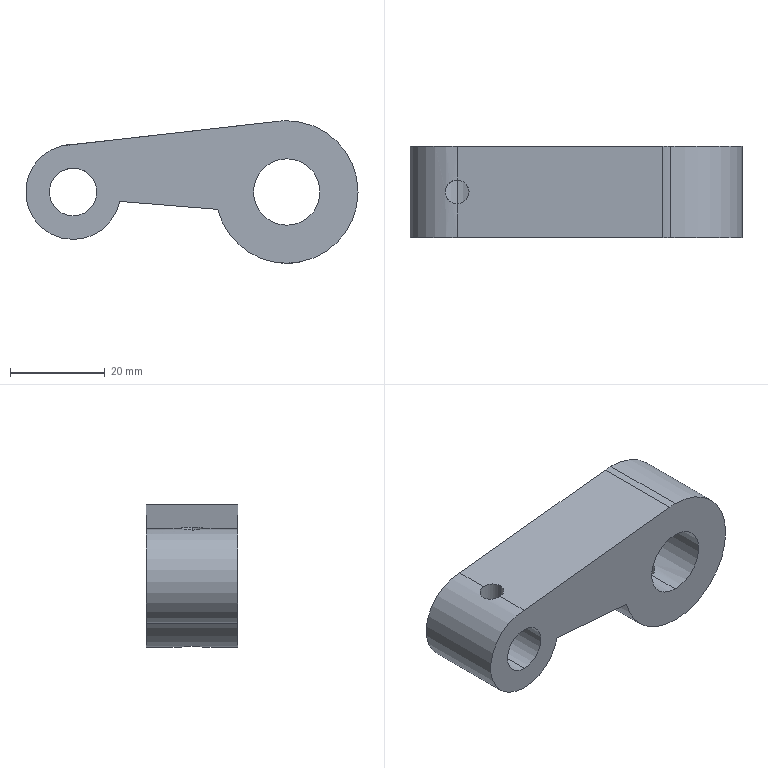Part | SolidWorks | features BaseBody 1 | 1 solid | 17 faces | box 70 x 19.2 x 30 mm | volume 21910 mm3 | cylinder 13 | plane 4 | commonest cylinder face diameters 5 x4 30 x3 10 x2 14 x2 20 x2
STEP:
#1=CARTESIAN_POINT('',(-45.,19.2,10.));
#2=VERTEX_POINT('',#1);
#3=CARTESIAN_POINT('',(-45.,19.2,-10.));
#4=VERTEX_POINT('',#3);
#5=CARTESIAN_POINT('',(-45.,19.2,0.));
#6=DIRECTION('',(0.,-1.,0.));
#7=DIRECTION('',(0.,0.,-1.));
#8=AXIS2_PLACEMENT_3D('',#5,#6,#7);
#9=CIRCLE('',#8,10.);
#10=EDGE_CURVE('',#2,#4,#9,.T.);
#11=ORIENTED_EDGE('',*,*,#10,.T.);
#12=CARTESIAN_POINT('',(-45.,0.,-10.));
#13=VERTEX_POINT('',#12);
#14=CARTESIAN_POINT('',(-45.,19.2,-10.));
#15=DIRECTION('',(0.,-1.,0.));
#16=VECTOR('',#15,1000.);
#17=LINE('',#14,#16);
#18=EDGE_CURVE('',#4,#13,#17,.T.);
#19=ORIENTED_EDGE('',*,*,#18,.T.);
#20=CARTESIAN_POINT('',(-45.,0.,10.));
#21=VERTEX_POINT('',#20);
#22=CARTESIAN_POINT('',(-45.,0.,0.));
#23=DIRECTION('',(0.,1.,0.));
#24=DIRECTION('',(0.,0.,-1.));
#25=AXIS2_PLACEMENT_3D('',#22,#23,#24);
#26=CIRCLE('',#25,10.);
#27=EDGE_CURVE('',#13,#21,#26,.T.);
#28=ORIENTED_EDGE('',*,*,#27,.T.);
#29=CARTESIAN_POINT('',(-45.,7.1,10.));
#30=VERTEX_POINT('',#29);
#31=CARTESIAN_POINT('',(-45.,19.2,10.));
#32=DIRECTION('',(0.,1.,0.));
#33=VECTOR('',#32,1000.);
#34=LINE('',#31,#33);
#35=EDGE_CURVE('',#21,#30,#34,.T.);
#36=ORIENTED_EDGE('',*,*,#35,.T.);
#37=CARTESIAN_POINT('',(-47.5,9.6,9.682));
#38=VERTEX_POINT('',#37);
#39=CARTESIAN_POINT('',(-45.,7.1,10.));
#40=CARTESIAN_POINT('',(-45.166,7.1,10.));
#41=CARTESIAN_POINT('',(-45.329,7.116,9.996));
#42=CARTESIAN_POINT('',(-45.649,7.18,9.98));
#43=CARTESIAN_POINT('',(-45.808,7.229,9.968));
#44=CARTESIAN_POINT('',(-46.11,7.354,9.939));
#45=CARTESIAN_POINT('',(-46.254,7.431,9.922));
#46=CARTESIAN_POINT('',(-46.525,7.612,9.884));
#47=CARTESIAN_POINT('',(-46.653,7.717,9.863));
#48=CARTESIAN_POINT('',(-46.997,8.061,9.801));
#49=CARTESIAN_POINT('',(-47.183,8.339,9.76));
#50=CARTESIAN_POINT('',(-47.37,8.789,9.715));
#51=CARTESIAN_POINT('',(-47.419,8.947,9.703));
#52=CARTESIAN_POINT('',(-47.484,9.27,9.687));
#53=CARTESIAN_POINT('',(-47.5,9.434,9.682));
#54=CARTESIAN_POINT('',(-47.5,9.6,9.682));
#55=B_SPLINE_CURVE_WITH_KNOTS('',3,(#39,#40,#41,#42,#43,#44,#45,#46,#47,#48,#49,#50,#51,#52,#53,#54),.UNSPECIFIED.,.F.,.F.,(4,2,2,2,2,2,2,4),(-0.003921,-0.003431,-0.002941,-0.002451,-0.00196,-0.0009802,-0.0004901,0.),.UNSPECIFIED.);
#56=EDGE_CURVE('',#30,#38,#55,.T.);
#57=ORIENTED_EDGE('',*,*,#56,.T.);
#58=CARTESIAN_POINT('',(-45.,12.1,10.));
#59=VERTEX_POINT('',#58);
#60=CARTESIAN_POINT('',(-47.5,9.6,9.682));
#61=CARTESIAN_POINT('',(-47.5,9.766,9.682));
#62=CARTESIAN_POINT('',(-47.484,9.929,9.687));
#63=CARTESIAN_POINT('',(-47.42,10.249,9.703));
#64=CARTESIAN_POINT('',(-47.372,10.408,9.715));
#65=CARTESIAN_POINT('',(-47.246,10.71,9.745));
#66=CARTESIAN_POINT('',(-47.169,10.853,9.762));
#67=CARTESIAN_POINT('',(-46.988,11.125,9.801));
#68=CARTESIAN_POINT('',(-46.883,11.252,9.822));
#69=CARTESIAN_POINT('',(-46.539,11.597,9.884));
#70=CARTESIAN_POINT('',(-46.261,11.783,9.925));
#71=CARTESIAN_POINT('',(-45.811,11.97,9.968));
#72=CARTESIAN_POINT('',(-45.653,12.019,9.98));
#73=CARTESIAN_POINT('',(-45.33,12.084,9.996));
#74=CARTESIAN_POINT('',(-45.166,12.1,10.));
#75=CARTESIAN_POINT('',(-45.,12.1,10.));
#76=B_SPLINE_CURVE_WITH_KNOTS('',3,(#60,#61,#62,#63,#64,#65,#66,#67,#68,#69,#70,#71,#72,#73,#74,#75),.UNSPECIFIED.,.F.,.F.,(4,2,2,2,2,2,2,4),(0.,0.0004901,0.0009802,0.00147,0.00196,0.002941,0.003431,0.003921),.UNSPECIFIED.);
#77=EDGE_CURVE('',#38,#59,#76,.T.);
#78=ORIENTED_EDGE('',*,*,#77,.T.);
#79=CARTESIAN_POINT('',(-45.,19.2,10.));
#80=DIRECTION('',(0.,1.,0.));
#81=VECTOR('',#80,1000.);
#82=LINE('',#79,#81);
#83=EDGE_CURVE('',#59,#2,#82,.T.);
#84=ORIENTED_EDGE('',*,*,#83,.T.);
#85=EDGE_LOOP('',(#11,#19,#28,#36,#57,#78,#84));
#86=FACE_OUTER_BOUND('',#85,.T.);
#87=CARTESIAN_POINT('',(-45.,19.2,0.));
#88=DIRECTION('',(0.,-1.,0.));
#89=DIRECTION('',(0.,0.,-1.));
#90=AXIS2_PLACEMENT_3D('',#87,#88,#89);
#91=CYLINDRICAL_SURFACE('',#90,10.);
#92=ADVANCED_FACE('',(#86),#91,.T.);
#93=CARTESIAN_POINT('',(0.,19.2,-15.));
#94=VERTEX_POINT('',#93);
#95=CARTESIAN_POINT('',(0.,19.2,15.));
#96=VERTEX_POINT('',#95);
#97=CARTESIAN_POINT('',(0.,19.2,0.));
#98=DIRECTION('',(0.,-1.,0.));
#99=DIRECTION('',(0.,0.,-1.));
#100=AXIS2_PLACEMENT_3D('',#97,#98,#99);
#101=CIRCLE('',#100,15.);
#102=EDGE_CURVE('',#94,#96,#101,.T.);
#103=ORIENTED_EDGE('',*,*,#102,.T.);
#104=CARTESIAN_POINT('',(0.,0.,15.));
#105=VERTEX_POINT('',#104);
#106=CARTESIAN_POINT('',(0.,19.2,15.));
#107=DIRECTION('',(0.,-1.,0.));
#108=VECTOR('',#107,1000.);
#109=LINE('',#106,#108);
#110=EDGE_CURVE('',#96,#105,#109,.T.);
#111=ORIENTED_EDGE('',*,*,#110,.T.);
#112=CARTESIAN_POINT('',(0.,0.,-15.));
#113=VERTEX_POINT('',#112);
#114=CARTESIAN_POINT('',(0.,0.,0.));
#115=DIRECTION('',(0.,1.,0.));
#116=DIRECTION('',(0.,0.,-1.));
#117=AXIS2_PLACEMENT_3D('',#114,#115,#116);
#118=CIRCLE('',#117,15.);
#119=EDGE_CURVE('',#105,#113,#118,.T.);
#120=ORIENTED_EDGE('',*,*,#119,.T.);
#121=CARTESIAN_POINT('',(0.,7.1,-15.));
#122=VERTEX_POINT('',#121);
#123=CARTESIAN_POINT('',(0.,19.2,-15.));
#124=DIRECTION('',(0.,-1.,0.));
#125=VECTOR('',#124,1000.);
#126=LINE('',#123,#125);
#127=EDGE_CURVE('',#122,#113,#126,.T.);
#128=ORIENTED_EDGE('',*,*,#127,.F.);
#129=CARTESIAN_POINT('',(2.5,9.6,-14.79));
#130=VERTEX_POINT('',#129);
#131=CARTESIAN_POINT('',(0.,7.1,-15.));
#132=CARTESIAN_POINT('',(0.1654,7.1,-15.));
#133=CARTESIAN_POINT('',(0.3279,7.116,-14.997));
#134=CARTESIAN_POINT('',(0.6477,7.18,-14.987));
#135=CARTESIAN_POINT('',(0.8065,7.228,-14.979));
#136=CARTESIAN_POINT('',(1.109,7.353,-14.96));
#137=CARTESIAN_POINT('',(1.252,7.43,-14.948));
#138=CARTESIAN_POINT('',(1.524,7.611,-14.923));
#139=CARTESIAN_POINT('',(1.652,7.717,-14.909));
#140=CARTESIAN_POINT('',(1.882,7.947,-14.882));
#141=CARTESIAN_POINT('',(1.986,8.072,-14.868));
#142=CARTESIAN_POINT('',(2.168,8.345,-14.843));
#143=CARTESIAN_POINT('',(2.246,8.49,-14.831));
#144=CARTESIAN_POINT('',(2.433,8.941,-14.802));
#145=CARTESIAN_POINT('',(2.5,9.269,-14.79));
#146=CARTESIAN_POINT('',(2.5,9.6,-14.79));
#147=B_SPLINE_CURVE_WITH_KNOTS('',3,(#131,#132,#133,#134,#135,#136,#137,#138,#139,#140,#141,#142,#143,#144,#145,#146),.UNSPECIFIED.,.F.,.F.,(4,2,2,2,2,2,2,4),(0.003912,0.004401,0.00489,0.005379,0.005868,0.006357,0.006846,0.007825),.UNSPECIFIED.);
#148=EDGE_CURVE('',#122,#130,#147,.T.);
#149=ORIENTED_EDGE('',*,*,#148,.T.);
#150=CARTESIAN_POINT('',(0.,12.1,-15.));
#151=VERTEX_POINT('',#150);
#152=CARTESIAN_POINT('',(2.5,9.6,-14.79));
#153=CARTESIAN_POINT('',(2.5,9.765,-14.79));
#154=CARTESIAN_POINT('',(2.484,9.928,-14.793));
#155=CARTESIAN_POINT('',(2.42,10.248,-14.804));
#156=CARTESIAN_POINT('',(2.372,10.407,-14.811));
#157=CARTESIAN_POINT('',(2.247,10.709,-14.831));
#158=CARTESIAN_POINT('',(2.17,10.852,-14.843));
#159=CARTESIAN_POINT('',(1.989,11.124,-14.868));
#160=CARTESIAN_POINT('',(1.883,11.252,-14.882));
#161=CARTESIAN_POINT('',(1.653,11.482,-14.909));
#162=CARTESIAN_POINT('',(1.528,11.586,-14.923));
#163=CARTESIAN_POINT('',(1.255,11.768,-14.948));
#164=CARTESIAN_POINT('',(1.11,11.846,-14.96));
#165=CARTESIAN_POINT('',(0.6593,12.033,-14.989));
#166=CARTESIAN_POINT('',(0.3308,12.1,-15.));
#167=CARTESIAN_POINT('',(0.,12.1,-15.));
#168=B_SPLINE_CURVE_WITH_KNOTS('',3,(#152,#153,#154,#155,#156,#157,#158,#159,#160,#161,#162,#163,#164,#165,#166,#167),.UNSPECIFIED.,.F.,.F.,(4,2,2,2,2,2,2,4),(0.007825,0.008314,0.008803,0.009292,0.009781,0.01027,0.01076,0.01174),.UNSPECIFIED.);
#169=EDGE_CURVE('',#130,#151,#168,.T.);
#170=ORIENTED_EDGE('',*,*,#169,.T.);
#171=CARTESIAN_POINT('',(0.,19.2,-15.));
#172=DIRECTION('',(0.,-1.,0.));
#173=VECTOR('',#172,1000.);
#174=LINE('',#171,#173);
#175=EDGE_CURVE('',#94,#151,#174,.T.);
#176=ORIENTED_EDGE('',*,*,#175,.F.);
#177=EDGE_LOOP('',(#103,#111,#120,#128,#149,#170,#176));
#178=FACE_OUTER_BOUND('',#177,.T.);
#179=CARTESIAN_POINT('',(0.,19.2,0.));
#180=DIRECTION('',(0.,-1.,0.));
#181=DIRECTION('',(0.,0.,-1.));
#182=AXIS2_PLACEMENT_3D('',#179,#180,#181);
#183=CYLINDRICAL_SURFACE('',#182,15.);
#184=ADVANCED_FACE('',(#178),#183,.T.);
#185=CARTESIAN_POINT('',(-14.547,19.2,-3.66));
#186=VERTEX_POINT('',#185);
#187=CARTESIAN_POINT('',(0.,19.2,0.));
#188=DIRECTION('',(0.,-1.,0.));
#189=DIRECTION('',(0.,0.,-1.));
#190=AXIS2_PLACEMENT_3D('',#187,#188,#189);
#191=CIRCLE('',#190,15.);
#192=EDGE_CURVE('',#186,#94,#191,.T.);
#193=ORIENTED_EDGE('',*,*,#192,.T.);
#194=ORIENTED_EDGE('',*,*,#175,.T.);
#195=CARTESIAN_POINT('',(-2.5,9.6,-14.79));
#196=VERTEX_POINT('',#195);
#197=CARTESIAN_POINT('',(0.,12.1,-15.));
#198=CARTESIAN_POINT('',(-0.1654,12.1,-15.));
#199=CARTESIAN_POINT('',(-0.3279,12.084,-14.997));
#200=CARTESIAN_POINT('',(-0.6477,12.02,-14.987));
#201=CARTESIAN_POINT('',(-0.8065,11.972,-14.979));
#202=CARTESIAN_POINT('',(-1.109,11.847,-14.96));
#203=CARTESIAN_POINT('',(-1.252,11.77,-14.948));
#204=CARTESIAN_POINT('',(-1.524,11.589,-14.923));
#205=CARTESIAN_POINT('',(-1.652,11.483,-14.909));
#206=CARTESIAN_POINT('',(-1.882,11.253,-14.882));
#207=CARTESIAN_POINT('',(-1.986,11.128,-14.868));
#208=CARTESIAN_POINT('',(-2.168,10.855,-14.843));
#209=CARTESIAN_POINT('',(-2.246,10.71,-14.831));
#210=CARTESIAN_POINT('',(-2.433,10.259,-14.802));
#211=CARTESIAN_POINT('',(-2.5,9.931,-14.79));
#212=CARTESIAN_POINT('',(-2.5,9.6,-14.79));
#213=B_SPLINE_CURVE_WITH_KNOTS('',3,(#197,#198,#199,#200,#201,#202,#203,#204,#205,#206,#207,#208,#209,#210,#211,#212),.UNSPECIFIED.,.F.,.F.,(4,2,2,2,2,2,2,4),(-0.003912,-0.003423,-0.002934,-0.002445,-0.001956,-0.001467,-0.000978,0.),.UNSPECIFIED.);
#214=EDGE_CURVE('',#151,#196,#213,.T.);
#215=ORIENTED_EDGE('',*,*,#214,.T.);
#216=CARTESIAN_POINT('',(-2.5,9.6,-14.79));
#217=CARTESIAN_POINT('',(-2.5,9.435,-14.79));
#218=CARTESIAN_POINT('',(-2.484,9.272,-14.793));
#219=CARTESIAN_POINT('',(-2.42,8.952,-14.804));
#220=CARTESIAN_POINT('',(-2.372,8.793,-14.811));
#221=CARTESIAN_POINT('',(-2.247,8.491,-14.831));
#222=CARTESIAN_POINT('',(-2.17,8.348,-14.843));
#223=CARTESIAN_POINT('',(-1.989,8.076,-14.868));
#224=CARTESIAN_POINT('',(-1.883,7.948,-14.882));
#225=CARTESIAN_POINT('',(-1.653,7.718,-14.909));
#226=CARTESIAN_POINT('',(-1.528,7.614,-14.923));
#227=CARTESIAN_POINT('',(-1.255,7.432,-14.948));
#228=CARTESIAN_POINT('',(-1.11,7.354,-14.96));
#229=CARTESIAN_POINT('',(-0.6593,7.167,-14.989));
#230=CARTESIAN_POINT('',(-0.3308,7.1,-15.));
#231=CARTESIAN_POINT('',(0.,7.1,-15.));
#232=B_SPLINE_CURVE_WITH_KNOTS('',3,(#216,#217,#218,#219,#220,#221,#222,#223,#224,#225,#226,#227,#228,#229,#230,#231),.UNSPECIFIED.,.F.,.F.,(4,2,2,2,2,2,2,4),(0.,0.000489,0.0009781,0.001467,0.001956,0.002445,0.002934,0.003912),.UNSPECIFIED.);
#233=EDGE_CURVE('',#196,#122,#232,.T.);
#234=ORIENTED_EDGE('',*,*,#233,.T.);
#235=ORIENTED_EDGE('',*,*,#127,.T.);
#236=CARTESIAN_POINT('',(-14.547,0.,-3.66));
#237=VERTEX_POINT('',#236);
#238=CARTESIAN_POINT('',(0.,0.,0.));
#239=DIRECTION('',(0.,1.,0.));
#240=DIRECTION('',(0.,0.,-1.));
#241=AXIS2_PLACEMENT_3D('',#238,#239,#240);
#242=CIRCLE('',#241,15.);
#243=EDGE_CURVE('',#113,#237,#242,.T.);
#244=ORIENTED_EDGE('',*,*,#243,.T.);
#245=CARTESIAN_POINT('',(-14.547,19.2,-3.66));
#246=DIRECTION('',(0.,1.,0.));
#247=VECTOR('',#246,1000.);
#248=LINE('',#245,#247);
#249=EDGE_CURVE('',#237,#186,#248,.T.);
#250=ORIENTED_EDGE('',*,*,#249,.T.);
#251=EDGE_LOOP('',(#193,#194,#215,#234,#235,#244,#250));
#252=FACE_OUTER_BOUND('',#251,.T.);
#253=CARTESIAN_POINT('',(0.,19.2,0.));
#254=DIRECTION('',(0.,-1.,0.));
#255=DIRECTION('',(0.,0.,-1.));
#256=AXIS2_PLACEMENT_3D('',#253,#254,#255);
#257=CYLINDRICAL_SURFACE('',#256,15.);
#258=ADVANCED_FACE('',(#252),#257,.T.);
#259=CARTESIAN_POINT('',(0.,0.,7.));
#260=VERTEX_POINT('',#259);
#261=CARTESIAN_POINT('',(0.,0.,-7.));
#262=VERTEX_POINT('',#261);
#263=CARTESIAN_POINT('',(0.,0.,0.));
#264=DIRECTION('',(0.,-1.,0.));
#265=DIRECTION('',(0.,0.,1.));
#266=AXIS2_PLACEMENT_3D('',#263,#264,#265);
#267=CIRCLE('',#266,7.);
#268=EDGE_CURVE('',#260,#262,#267,.T.);
#269=ORIENTED_EDGE('',*,*,#268,.T.);
#270=CARTESIAN_POINT('',(0.,7.1,-7.));
#271=VERTEX_POINT('',#270);
#272=CARTESIAN_POINT('',(0.,0.,-7.));
#273=DIRECTION('',(0.,1.,0.));
#274=VECTOR('',#273,1000.);
#275=LINE('',#272,#274);
#276=EDGE_CURVE('',#262,#271,#275,.T.);
#277=ORIENTED_EDGE('',*,*,#276,.T.);
#278=CARTESIAN_POINT('',(-2.5,9.6,-6.538));
#279=VERTEX_POINT('',#278);
#280=CARTESIAN_POINT('',(-2.5,9.6,-6.538));
#281=CARTESIAN_POINT('',(-2.5,9.433,-6.538));
#282=CARTESIAN_POINT('',(-2.484,9.27,-6.545));
#283=CARTESIAN_POINT('',(-2.419,8.949,-6.569));
#284=CARTESIAN_POINT('',(-2.371,8.789,-6.587));
#285=CARTESIAN_POINT('',(-2.245,8.488,-6.631));
#286=CARTESIAN_POINT('',(-2.168,8.345,-6.656));
#287=CARTESIAN_POINT('',(-1.987,8.074,-6.713));
#288=CARTESIAN_POINT('',(-1.883,7.947,-6.743));
#289=CARTESIAN_POINT('',(-1.54,7.604,-6.833));
#290=CARTESIAN_POINT('',(-1.264,7.419,-6.892));
#291=CARTESIAN_POINT('',(-0.8135,7.23,-6.954));
#292=CARTESIAN_POINT('',(-0.6548,7.182,-6.971));
#293=CARTESIAN_POINT('',(-0.3308,7.116,-6.994));
#294=CARTESIAN_POINT('',(-0.1666,7.1,-7.));
#295=CARTESIAN_POINT('',(0.,7.1,-7.));
#296=B_SPLINE_CURVE_WITH_KNOTS('',3,(#280,#281,#282,#283,#284,#285,#286,#287,#288,#289,#290,#291,#292,#293,#294,#295),.UNSPECIFIED.,.F.,.F.,(4,2,2,2,2,2,2,4),(0.007876,0.008369,0.008861,0.009353,0.009846,0.01083,0.01132,0.01181),.UNSPECIFIED.);
#297=EDGE_CURVE('',#279,#271,#296,.T.);
#298=ORIENTED_EDGE('',*,*,#297,.F.);
#299=CARTESIAN_POINT('',(0.,12.1,-7.));
#300=VERTEX_POINT('',#299);
#301=CARTESIAN_POINT('',(0.,12.1,-7.));
#302=CARTESIAN_POINT('',(-0.1666,12.1,-7.));
#303=CARTESIAN_POINT('',(-0.3301,12.084,-6.994));
#304=CARTESIAN_POINT('',(-0.6514,12.019,-6.971));
#305=CARTESIAN_POINT('',(-0.8108,11.971,-6.955));
#306=CARTESIAN_POINT('',(-1.113,11.845,-6.913));
#307=CARTESIAN_POINT('',(-1.256,11.768,-6.888));
#308=CARTESIAN_POINT('',(-1.527,11.586,-6.833));
#309=CARTESIAN_POINT('',(-1.654,11.482,-6.803));
#310=CARTESIAN_POINT('',(-1.996,11.139,-6.713));
#311=CARTESIAN_POINT('',(-2.182,10.863,-6.653));
#312=CARTESIAN_POINT('',(-2.37,10.413,-6.587));
#313=CARTESIAN_POINT('',(-2.418,10.255,-6.569));
#314=CARTESIAN_POINT('',(-2.484,9.931,-6.545));
#315=CARTESIAN_POINT('',(-2.5,9.767,-6.538));
#316=CARTESIAN_POINT('',(-2.5,9.6,-6.538));
#317=B_SPLINE_CURVE_WITH_KNOTS('',3,(#301,#302,#303,#304,#305,#306,#307,#308,#309,#310,#311,#312,#313,#314,#315,#316),.UNSPECIFIED.,.F.,.F.,(4,2,2,2,2,2,2,4),(0.003938,0.004431,0.004923,0.005415,0.005907,0.006892,0.007384,0.007876),.UNSPECIFIED.);
#318=EDGE_CURVE('',#300,#279,#317,.T.);
#319=ORIENTED_EDGE('',*,*,#318,.F.);
#320=CARTESIAN_POINT('',(0.,19.2,-7.));
#321=VERTEX_POINT('',#320);
#322=CARTESIAN_POINT('',(0.,0.,-7.));
#323=DIRECTION('',(0.,1.,0.));
#324=VECTOR('',#323,1000.);
#325=LINE('',#322,#324);
#326=EDGE_CURVE('',#300,#321,#325,.T.);
#327=ORIENTED_EDGE('',*,*,#326,.T.);
#328=CARTESIAN_POINT('',(0.,19.2,7.));
#329=VERTEX_POINT('',#328);
#330=CARTESIAN_POINT('',(0.,19.2,0.));
#331=DIRECTION('',(0.,-1.,0.));
#332=DIRECTION('',(0.,0.,1.));
#333=AXIS2_PLACEMENT_3D('',#330,#331,#332);
#334=CIRCLE('',#333,7.);
#335=EDGE_CURVE('',#329,#321,#334,.T.);
#336=ORIENTED_EDGE('',*,*,#335,.F.);
#337=CARTESIAN_POINT('',(0.,0.,7.));
#338=DIRECTION('',(0.,1.,0.));
#339=VECTOR('',#338,1000.);
#340=LINE('',#337,#339);
#341=EDGE_CURVE('',#260,#329,#340,.T.);
#342=ORIENTED_EDGE('',*,*,#341,.F.);
#343=EDGE_LOOP('',(#269,#277,#298,#319,#327,#336,#342));
#344=FACE_OUTER_BOUND('',#343,.T.);
#345=CARTESIAN_POINT('',(0.,0.,0.));
#346=DIRECTION('',(0.,1.,0.));
#347=DIRECTION('',(0.,0.,1.));
#348=AXIS2_PLACEMENT_3D('',#345,#346,#347);
#349=CYLINDRICAL_SURFACE('',#348,7.);
#350=ADVANCED_FACE('',(#344),#349,.F.);
#351=CARTESIAN_POINT('',(-45.,0.,5.));
#352=VERTEX_POINT('',#351);
#353=CARTESIAN_POINT('',(-45.,0.,-5.));
#354=VERTEX_POINT('',#353);
#355=CARTESIAN_POINT('',(-45.,0.,0.));
#356=DIRECTION('',(0.,-1.,0.));
#357=DIRECTION('',(0.,0.,1.));
#358=AXIS2_PLACEMENT_3D('',#355,#356,#357);
#359=CIRCLE('',#358,5.);
#360=EDGE_CURVE('',#352,#354,#359,.T.);
#361=ORIENTED_EDGE('',*,*,#360,.T.);
#362=CARTESIAN_POINT('',(-45.,19.2,-5.));
#363=VERTEX_POINT('',#362);
#364=CARTESIAN_POINT('',(-45.,0.,-5.));
#365=DIRECTION('',(0.,1.,0.));
#366=VECTOR('',#365,1000.);
#367=LINE('',#364,#366);
#368=EDGE_CURVE('',#354,#363,#367,.T.);
#369=ORIENTED_EDGE('',*,*,#368,.T.);
#370=CARTESIAN_POINT('',(-45.,19.2,5.));
#371=VERTEX_POINT('',#370);
#372=CARTESIAN_POINT('',(-45.,19.2,0.));
#373=DIRECTION('',(0.,-1.,0.));
#374=DIRECTION('',(0.,0.,1.));
#375=AXIS2_PLACEMENT_3D('',#372,#373,#374);
#376=CIRCLE('',#375,5.);
#377=EDGE_CURVE('',#371,#363,#376,.T.);
#378=ORIENTED_EDGE('',*,*,#377,.F.);
#379=CARTESIAN_POINT('',(-45.,12.1,5.));
#380=VERTEX_POINT('',#379);
#381=CARTESIAN_POINT('',(-45.,0.,5.));
#382=DIRECTION('',(0.,1.,0.));
#383=VECTOR('',#382,1000.);
#384=LINE('',#381,#383);
#385=EDGE_CURVE('',#380,#371,#384,.T.);
#386=ORIENTED_EDGE('',*,*,#385,.F.);
#387=CARTESIAN_POINT('',(-47.5,9.6,4.33));
#388=VERTEX_POINT('',#387);
#389=CARTESIAN_POINT('',(-47.5,9.6,4.33));
#390=CARTESIAN_POINT('',(-47.5,9.768,4.33));
#391=CARTESIAN_POINT('',(-47.483,9.933,4.34));
#392=CARTESIAN_POINT('',(-47.418,10.256,4.377));
#393=CARTESIAN_POINT('',(-47.369,10.416,4.404));
#394=CARTESIAN_POINT('',(-47.18,10.867,4.502));
#395=CARTESIAN_POINT('',(-46.995,11.14,4.591));
#396=CARTESIAN_POINT('',(-46.656,11.48,4.719));
#397=CARTESIAN_POINT('',(-46.531,11.583,4.762));
#398=CARTESIAN_POINT('',(-46.261,11.765,4.84));
#399=CARTESIAN_POINT('',(-46.119,11.842,4.876));
#400=CARTESIAN_POINT('',(-45.819,11.968,4.935));
#401=CARTESIAN_POINT('',(-45.659,12.017,4.959));
#402=CARTESIAN_POINT('',(-45.334,12.083,4.992));
#403=CARTESIAN_POINT('',(-45.168,12.1,5.));
#404=CARTESIAN_POINT('',(-45.,12.1,5.));
#405=B_SPLINE_CURVE_WITH_KNOTS('',3,(#389,#390,#391,#392,#393,#394,#395,#396,#397,#398,#399,#400,#401,#402,#403,#404),.UNSPECIFIED.,.F.,.F.,(4,2,2,2,2,2,2,4),(0.007947,0.008443,0.00894,0.009933,0.01043,0.01093,0.01142,0.01192),.UNSPECIFIED.);
#406=EDGE_CURVE('',#388,#380,#405,.T.);
#407=ORIENTED_EDGE('',*,*,#406,.F.);
#408=CARTESIAN_POINT('',(-45.,7.1,5.));
#409=VERTEX_POINT('',#408);
#410=CARTESIAN_POINT('',(-45.,7.1,5.));
#411=CARTESIAN_POINT('',(-45.168,7.1,5.));
#412=CARTESIAN_POINT('',(-45.333,7.117,4.992));
#413=CARTESIAN_POINT('',(-45.657,7.182,4.959));
#414=CARTESIAN_POINT('',(-45.817,7.232,4.935));
#415=CARTESIAN_POINT('',(-46.27,7.422,4.846));
#416=CARTESIAN_POINT('',(-46.543,7.607,4.762));
#417=CARTESIAN_POINT('',(-46.882,7.947,4.634));
#418=CARTESIAN_POINT('',(-46.986,8.072,4.59));
#419=CARTESIAN_POINT('',(-47.166,8.341,4.508));
#420=CARTESIAN_POINT('',(-47.242,8.483,4.47));
#421=CARTESIAN_POINT('',(-47.368,8.782,4.404));
#422=CARTESIAN_POINT('',(-47.417,8.942,4.377));
#423=CARTESIAN_POINT('',(-47.483,9.267,4.34));
#424=CARTESIAN_POINT('',(-47.5,9.432,4.33));
#425=CARTESIAN_POINT('',(-47.5,9.6,4.33));
#426=B_SPLINE_CURVE_WITH_KNOTS('',3,(#410,#411,#412,#413,#414,#415,#416,#417,#418,#419,#420,#421,#422,#423,#424,#425),.UNSPECIFIED.,.F.,.F.,(4,2,2,2,2,2,2,4),(0.003974,0.004471,0.004967,0.00596,0.006457,0.006954,0.00745,0.007947),.UNSPECIFIED.);
#427=EDGE_CURVE('',#409,#388,#426,.T.);
#428=ORIENTED_EDGE('',*,*,#427,.F.);
#429=CARTESIAN_POINT('',(-45.,0.,5.));
#430=DIRECTION('',(0.,1.,0.));
#431=VECTOR('',#430,1000.);
#432=LINE('',#429,#431);
#433=EDGE_CURVE('',#352,#409,#432,.T.);
#434=ORIENTED_EDGE('',*,*,#433,.F.);
#435=EDGE_LOOP('',(#361,#369,#378,#386,#407,#428,#434));
#436=FACE_OUTER_BOUND('',#435,.T.);
#437=CARTESIAN_POINT('',(-45.,0.,0.));
#438=DIRECTION('',(0.,1.,0.));
#439=DIRECTION('',(0.,0.,1.));
#440=AXIS2_PLACEMENT_3D('',#437,#438,#439);
#441=CYLINDRICAL_SURFACE('',#440,5.);
#442=ADVANCED_FACE('',(#436),#441,.F.);
#443=ORIENTED_EDGE('',*,*,#233,.F.);
#444=CARTESIAN_POINT('',(-2.5,9.6,0.));
#445=DIRECTION('',(0.,0.,1.));
#446=VECTOR('',#445,1000.);
#447=LINE('',#444,#446);
#448=EDGE_CURVE('',#196,#279,#447,.T.);
#449=ORIENTED_EDGE('',*,*,#448,.T.);
#450=ORIENTED_EDGE('',*,*,#297,.T.);
#451=CARTESIAN_POINT('',(2.5,9.6,-6.538));
#452=VERTEX_POINT('',#451);
#453=CARTESIAN_POINT('',(0.,7.1,-7.));
#454=CARTESIAN_POINT('',(0.1666,7.1,-7.));
#455=CARTESIAN_POINT('',(0.3301,7.116,-6.994));
#456=CARTESIAN_POINT('',(0.6514,7.181,-6.971));
#457=CARTESIAN_POINT('',(0.8108,7.229,-6.955));
#458=CARTESIAN_POINT('',(1.113,7.355,-6.913));
#459=CARTESIAN_POINT('',(1.256,7.432,-6.888));
#460=CARTESIAN_POINT('',(1.527,7.614,-6.833));
#461=CARTESIAN_POINT('',(1.654,7.718,-6.803));
#462=CARTESIAN_POINT('',(1.996,8.061,-6.713));
#463=CARTESIAN_POINT('',(2.182,8.337,-6.653));
#464=CARTESIAN_POINT('',(2.37,8.787,-6.587));
#465=CARTESIAN_POINT('',(2.418,8.945,-6.569));
#466=CARTESIAN_POINT('',(2.484,9.269,-6.545));
#467=CARTESIAN_POINT('',(2.5,9.433,-6.538));
#468=CARTESIAN_POINT('',(2.5,9.6,-6.538));
#469=B_SPLINE_CURVE_WITH_KNOTS('',3,(#453,#454,#455,#456,#457,#458,#459,#460,#461,#462,#463,#464,#465,#466,#467,#468),.UNSPECIFIED.,.F.,.F.,(4,2,2,2,2,2,2,4),(-0.003938,-0.003446,-0.002954,-0.002461,-0.001969,-0.0009845,-0.0004923,0.),.UNSPECIFIED.);
#470=EDGE_CURVE('',#271,#452,#469,.T.);
#471=ORIENTED_EDGE('',*,*,#470,.T.);
#472=CARTESIAN_POINT('',(2.5,9.6,0.));
#473=DIRECTION('',(0.,0.,1.));
#474=VECTOR('',#473,1000.);
#475=LINE('',#472,#474);
#476=EDGE_CURVE('',#130,#452,#475,.T.);
#477=ORIENTED_EDGE('',*,*,#476,.F.);
#478=ORIENTED_EDGE('',*,*,#148,.F.);
#479=EDGE_LOOP('',(#443,#449,#450,#471,#477,#478));
#480=FACE_OUTER_BOUND('',#479,.T.);
#481=CARTESIAN_POINT('',(0.,9.6,0.));
#482=DIRECTION('',(0.,0.,1.));
#483=DIRECTION('',(1.,0.,0.));
#484=AXIS2_PLACEMENT_3D('',#481,#482,#483);
#485=CYLINDRICAL_SURFACE('',#484,2.5);
#486=ADVANCED_FACE('',(#480),#485,.F.);
#487=CARTESIAN_POINT('',(-42.5,9.6,10.283));
#488=VERTEX_POINT('',#487);
#489=CARTESIAN_POINT('',(-45.,7.1,10.));
#490=CARTESIAN_POINT('',(-43.536,7.1,10.166));
#491=CARTESIAN_POINT('',(-42.5,8.136,10.283));
#492=CARTESIAN_POINT('',(-42.5,9.6,10.283));
#493=(BOUNDED_CURVE()B_SPLINE_CURVE(3,(#489,#490,#491,#492),.UNSPECIFIED.,.F.,.F.)B_SPLINE_CURVE_WITH_KNOTS((4,4),(1.571,3.142),.UNSPECIFIED.)CURVE()GEOMETRIC_REPRESENTATION_ITEM()RATIONAL_B_SPLINE_CURVE((1.,0.8047,0.8047,1.))REPRESENTATION_ITEM(''));
#494=EDGE_CURVE('',#30,#488,#493,.T.);
#495=ORIENTED_EDGE('',*,*,#494,.T.);
#496=CARTESIAN_POINT('',(-42.5,9.6,4.33));
#497=VERTEX_POINT('',#496);
#498=CARTESIAN_POINT('',(-42.5,9.6,0.));
#499=DIRECTION('',(0.,0.,-1.));
#500=VECTOR('',#499,1000.);
#501=LINE('',#498,#500);
#502=EDGE_CURVE('',#488,#497,#501,.T.);
#503=ORIENTED_EDGE('',*,*,#502,.T.);
#504=CARTESIAN_POINT('',(-42.5,9.6,4.33));
#505=CARTESIAN_POINT('',(-42.5,9.432,4.33));
#506=CARTESIAN_POINT('',(-42.517,9.267,4.34));
#507=CARTESIAN_POINT('',(-42.582,8.944,4.377));
#508=CARTESIAN_POINT('',(-42.631,8.784,4.404));
#509=CARTESIAN_POINT('',(-42.82,8.333,4.502));
#510=CARTESIAN_POINT('',(-43.005,8.06,4.591));
#511=CARTESIAN_POINT('',(-43.344,7.72,4.719));
#512=CARTESIAN_POINT('',(-43.469,7.617,4.762));
#513=CARTESIAN_POINT('',(-43.739,7.435,4.84));
#514=CARTESIAN_POINT('',(-43.881,7.358,4.876));
#515=CARTESIAN_POINT('',(-44.181,7.232,4.935));
#516=CARTESIAN_POINT('',(-44.341,7.183,4.959));
#517=CARTESIAN_POINT('',(-44.666,7.117,4.992));
#518=CARTESIAN_POINT('',(-44.832,7.1,5.));
#519=CARTESIAN_POINT('',(-45.,7.1,5.));
#520=B_SPLINE_CURVE_WITH_KNOTS('',3,(#504,#505,#506,#507,#508,#509,#510,#511,#512,#513,#514,#515,#516,#517,#518,#519),.UNSPECIFIED.,.F.,.F.,(4,2,2,2,2,2,2,4),(0.,0.0004967,0.0009935,0.001987,0.002484,0.00298,0.003477,0.003974),.UNSPECIFIED.);
#521=EDGE_CURVE('',#497,#409,#520,.T.);
#522=ORIENTED_EDGE('',*,*,#521,.T.);
#523=ORIENTED_EDGE('',*,*,#427,.T.);
#524=CARTESIAN_POINT('',(-47.5,9.6,0.));
#525=DIRECTION('',(0.,0.,-1.));
#526=VECTOR('',#525,1000.);
#527=LINE('',#524,#526);
#528=EDGE_CURVE('',#38,#388,#527,.T.);
#529=ORIENTED_EDGE('',*,*,#528,.F.);
#530=ORIENTED_EDGE('',*,*,#56,.F.);
#531=EDGE_LOOP('',(#495,#503,#522,#523,#529,#530));
#532=FACE_OUTER_BOUND('',#531,.T.);
#533=CARTESIAN_POINT('',(-45.,9.6,0.));
#534=DIRECTION('',(0.,0.,-1.));
#535=DIRECTION('',(-1.,0.,0.));
#536=AXIS2_PLACEMENT_3D('',#533,#534,#535);
#537=CYLINDRICAL_SURFACE('',#536,2.5);
#538=ADVANCED_FACE('',(#532),#537,.F.);
#539=CARTESIAN_POINT('',(-35.197,0.,-1.973));
#540=VERTEX_POINT('',#539);
#541=CARTESIAN_POINT('',(-14.547,0.,-3.66));
#542=DIRECTION('',(-0.9967,0.,0.08143));
#543=VECTOR('',#542,1000.);
#544=LINE('',#541,#543);
#545=EDGE_CURVE('',#237,#540,#544,.T.);
#546=ORIENTED_EDGE('',*,*,#545,.F.);
#547=ORIENTED_EDGE('',*,*,#243,.F.);
#548=ORIENTED_EDGE('',*,*,#119,.F.);
#549=CARTESIAN_POINT('',(-1.688,0.,14.905));
#550=VERTEX_POINT('',#549);
#551=CARTESIAN_POINT('',(0.,0.,0.));
#552=DIRECTION('',(0.,1.,0.));
#553=DIRECTION('',(0.,0.,-1.));
#554=AXIS2_PLACEMENT_3D('',#551,#552,#553);
#555=CIRCLE('',#554,15.);
#556=EDGE_CURVE('',#550,#105,#555,.T.);
#557=ORIENTED_EDGE('',*,*,#556,.F.);
#558=CARTESIAN_POINT('',(-45.,0.,10.));
#559=DIRECTION('',(0.9936,0.,0.1125));
#560=VECTOR('',#559,1000.);
#561=LINE('',#558,#560);
#562=EDGE_CURVE('',#21,#550,#561,.T.);
#563=ORIENTED_EDGE('',*,*,#562,.F.);
#564=ORIENTED_EDGE('',*,*,#27,.F.);
#565=CARTESIAN_POINT('',(-45.,0.,0.));
#566=DIRECTION('',(0.,1.,0.));
#567=DIRECTION('',(0.,0.,-1.));
#568=AXIS2_PLACEMENT_3D('',#565,#566,#567);
#569=CIRCLE('',#568,10.);
#570=EDGE_CURVE('',#540,#13,#569,.T.);
#571=ORIENTED_EDGE('',*,*,#570,.F.);
#572=EDGE_LOOP('',(#546,#547,#548,#557,#563,#564,#571));
#573=FACE_OUTER_BOUND('',#572,.T.);
#574=ORIENTED_EDGE('',*,*,#268,.F.);
#575=CARTESIAN_POINT('',(0.,0.,0.));
#576=DIRECTION('',(0.,-1.,0.));
#577=DIRECTION('',(0.,0.,1.));
#578=AXIS2_PLACEMENT_3D('',#575,#576,#577);
#579=CIRCLE('',#578,7.);
#580=EDGE_CURVE('',#262,#260,#579,.T.);
#581=ORIENTED_EDGE('',*,*,#580,.F.);
#582=EDGE_LOOP('',(#574,#581));
#583=FACE_BOUND('',#582,.T.);
#584=ORIENTED_EDGE('',*,*,#360,.F.);
#585=CARTESIAN_POINT('',(-45.,0.,0.));
#586=DIRECTION('',(0.,-1.,0.));
#587=DIRECTION('',(0.,0.,1.));
#588=AXIS2_PLACEMENT_3D('',#585,#586,#587);
#589=CIRCLE('',#588,5.);
#590=EDGE_CURVE('',#354,#352,#589,.T.);
#591=ORIENTED_EDGE('',*,*,#590,.F.);
#592=EDGE_LOOP('',(#584,#591));
#593=FACE_BOUND('',#592,.T.);
#594=CARTESIAN_POINT('',(-45.,0.,0.));
#595=DIRECTION('',(0.,1.,0.));
#596=DIRECTION('',(0.,0.,1.));
#597=AXIS2_PLACEMENT_3D('',#594,#595,#596);
#598=PLANE('',#597);
#599=ADVANCED_FACE('',(#573,#583,#593),#598,.F.);
#600=ORIENTED_EDGE('',*,*,#18,.F.);
#601=CARTESIAN_POINT('',(-35.197,19.2,-1.973));
#602=VERTEX_POINT('',#601);
#603=CARTESIAN_POINT('',(-45.,19.2,0.));
#604=DIRECTION('',(0.,-1.,0.));
#605=DIRECTION('',(0.,0.,-1.));
#606=AXIS2_PLACEMENT_3D('',#603,#604,#605);
#607=CIRCLE('',#606,10.);
#608=EDGE_CURVE('',#4,#602,#607,.T.);
#609=ORIENTED_EDGE('',*,*,#608,.T.);
#610=CARTESIAN_POINT('',(-35.197,19.2,-1.973));
#611=DIRECTION('',(0.,-1.,0.));
#612=VECTOR('',#611,1000.);
#613=LINE('',#610,#612);
#614=EDGE_CURVE('',#602,#540,#613,.T.);
#615=ORIENTED_EDGE('',*,*,#614,.T.);
#616=ORIENTED_EDGE('',*,*,#570,.T.);
#617=EDGE_LOOP('',(#600,#609,#615,#616));
#618=FACE_OUTER_BOUND('',#617,.T.);
#619=CARTESIAN_POINT('',(-45.,19.2,0.));
#620=DIRECTION('',(0.,-1.,0.));
#621=DIRECTION('',(0.,0.,-1.));
#622=AXIS2_PLACEMENT_3D('',#619,#620,#621);
#623=CYLINDRICAL_SURFACE('',#622,10.);
#624=ADVANCED_FACE('',(#618),#623,.T.);
#625=ORIENTED_EDGE('',*,*,#614,.F.);
#626=CARTESIAN_POINT('',(-14.547,19.2,-3.66));
#627=DIRECTION('',(-0.9967,0.,0.08143));
#628=VECTOR('',#627,1000.);
#629=LINE('',#626,#628);
#630=EDGE_CURVE('',#186,#602,#629,.T.);
#631=ORIENTED_EDGE('',*,*,#630,.F.);
#632=ORIENTED_EDGE('',*,*,#249,.F.);
#633=ORIENTED_EDGE('',*,*,#545,.T.);
#634=EDGE_LOOP('',(#625,#631,#632,#633));
#635=FACE_OUTER_BOUND('',#634,.T.);
#636=CARTESIAN_POINT('',(-14.547,19.2,-3.66));
#637=DIRECTION('',(0.08143,0.,0.9967));
#638=DIRECTION('',(0.9967,0.,-0.08143));
#639=AXIS2_PLACEMENT_3D('',#636,#637,#638);
#640=PLANE('',#639);
#641=ADVANCED_FACE('',(#635),#640,.F.);
#642=ORIENTED_EDGE('',*,*,#110,.F.);
#643=CARTESIAN_POINT('',(-1.688,19.2,14.905));
#644=VERTEX_POINT('',#643);
#645=CARTESIAN_POINT('',(0.,19.2,0.));
#646=DIRECTION('',(0.,-1.,0.));
#647=DIRECTION('',(0.,0.,-1.));
#648=AXIS2_PLACEMENT_3D('',#645,#646,#647);
#649=CIRCLE('',#648,15.);
#650=EDGE_CURVE('',#96,#644,#649,.T.);
#651=ORIENTED_EDGE('',*,*,#650,.T.);
#652=CARTESIAN_POINT('',(-1.688,19.2,14.905));
#653=DIRECTION('',(0.,-1.,0.));
#654=VECTOR('',#653,1000.);
#655=LINE('',#652,#654);
#656=EDGE_CURVE('',#644,#550,#655,.T.);
#657=ORIENTED_EDGE('',*,*,#656,.T.);
#658=ORIENTED_EDGE('',*,*,#556,.T.);
#659=EDGE_LOOP('',(#642,#651,#657,#658));
#660=FACE_OUTER_BOUND('',#659,.T.);
#661=CARTESIAN_POINT('',(0.,19.2,0.));
#662=DIRECTION('',(0.,-1.,0.));
#663=DIRECTION('',(0.,0.,-1.));
#664=AXIS2_PLACEMENT_3D('',#661,#662,#663);
#665=CYLINDRICAL_SURFACE('',#664,15.);
#666=ADVANCED_FACE('',(#660),#665,.T.);
#667=ORIENTED_EDGE('',*,*,#494,.F.);
#668=ORIENTED_EDGE('',*,*,#35,.F.);
#669=ORIENTED_EDGE('',*,*,#562,.T.);
#670=ORIENTED_EDGE('',*,*,#656,.F.);
#671=CARTESIAN_POINT('',(-45.,19.2,10.));
#672=DIRECTION('',(0.9936,0.,0.1125));
#673=VECTOR('',#672,1000.);
#674=LINE('',#671,#673);
#675=EDGE_CURVE('',#2,#644,#674,.T.);
#676=ORIENTED_EDGE('',*,*,#675,.F.);
#677=ORIENTED_EDGE('',*,*,#83,.F.);
#678=CARTESIAN_POINT('',(-42.5,9.6,10.283));
#679=CARTESIAN_POINT('',(-42.5,11.064,10.283));
#680=CARTESIAN_POINT('',(-43.536,12.1,10.166));
#681=CARTESIAN_POINT('',(-45.,12.1,10.));
#682=(BOUNDED_CURVE()B_SPLINE_CURVE(3,(#678,#679,#680,#681),.UNSPECIFIED.,.F.,.F.)B_SPLINE_CURVE_WITH_KNOTS((4,4),(3.142,4.712),.UNSPECIFIED.)CURVE()GEOMETRIC_REPRESENTATION_ITEM()RATIONAL_B_SPLINE_CURVE((1.,0.8047,0.8047,1.))REPRESENTATION_ITEM(''));
#683=EDGE_CURVE('',#488,#59,#682,.T.);
#684=ORIENTED_EDGE('',*,*,#683,.F.);
#685=EDGE_LOOP('',(#667,#668,#669,#670,#676,#677,#684));
#686=FACE_OUTER_BOUND('',#685,.T.);
#687=CARTESIAN_POINT('',(-45.,19.2,10.));
#688=DIRECTION('',(0.1125,0.,-0.9936));
#689=DIRECTION('',(-0.9936,0.,-0.1125));
#690=AXIS2_PLACEMENT_3D('',#687,#688,#689);
#691=PLANE('',#690);
#692=ADVANCED_FACE('',(#686),#691,.F.);
#693=ORIENTED_EDGE('',*,*,#276,.F.);
#694=ORIENTED_EDGE('',*,*,#580,.T.);
#695=ORIENTED_EDGE('',*,*,#341,.T.);
#696=CARTESIAN_POINT('',(0.,19.2,0.));
#697=DIRECTION('',(0.,-1.,0.));
#698=DIRECTION('',(0.,0.,1.));
#699=AXIS2_PLACEMENT_3D('',#696,#697,#698);
#700=CIRCLE('',#699,7.);
#701=EDGE_CURVE('',#321,#329,#700,.T.);
#702=ORIENTED_EDGE('',*,*,#701,.F.);
#703=ORIENTED_EDGE('',*,*,#326,.F.);
#704=CARTESIAN_POINT('',(2.5,9.6,-6.538));
#705=CARTESIAN_POINT('',(2.5,9.767,-6.538));
#706=CARTESIAN_POINT('',(2.484,9.93,-6.545));
#707=CARTESIAN_POINT('',(2.419,10.251,-6.569));
#708=CARTESIAN_POINT('',(2.371,10.411,-6.587));
#709=CARTESIAN_POINT('',(2.245,10.712,-6.631));
#710=CARTESIAN_POINT('',(2.168,10.855,-6.656));
#711=CARTESIAN_POINT('',(1.987,11.126,-6.713));
#712=CARTESIAN_POINT('',(1.883,11.253,-6.743));
#713=CARTESIAN_POINT('',(1.54,11.596,-6.833));
#714=CARTESIAN_POINT('',(1.264,11.781,-6.892));
#715=CARTESIAN_POINT('',(0.8135,11.97,-6.954));
#716=CARTESIAN_POINT('',(0.6548,12.018,-6.971));
#717=CARTESIAN_POINT('',(0.3308,12.084,-6.994));
#718=CARTESIAN_POINT('',(0.1666,12.1,-7.));
#719=CARTESIAN_POINT('',(0.,12.1,-7.));
#720=B_SPLINE_CURVE_WITH_KNOTS('',3,(#704,#705,#706,#707,#708,#709,#710,#711,#712,#713,#714,#715,#716,#717,#718,#719),.UNSPECIFIED.,.F.,.F.,(4,2,2,2,2,2,2,4),(0.,0.0004923,0.0009846,0.001477,0.001969,0.002954,0.003446,0.003938),.UNSPECIFIED.);
#721=EDGE_CURVE('',#452,#300,#720,.T.);
#722=ORIENTED_EDGE('',*,*,#721,.F.);
#723=ORIENTED_EDGE('',*,*,#470,.F.);
#724=EDGE_LOOP('',(#693,#694,#695,#702,#703,#722,#723));
#725=FACE_OUTER_BOUND('',#724,.T.);
#726=CARTESIAN_POINT('',(0.,0.,0.));
#727=DIRECTION('',(0.,1.,0.));
#728=DIRECTION('',(0.,0.,1.));
#729=AXIS2_PLACEMENT_3D('',#726,#727,#728);
#730=CYLINDRICAL_SURFACE('',#729,7.);
#731=ADVANCED_FACE('',(#725),#730,.F.);
#732=ORIENTED_EDGE('',*,*,#368,.F.);
#733=ORIENTED_EDGE('',*,*,#590,.T.);
#734=ORIENTED_EDGE('',*,*,#433,.T.);
#735=ORIENTED_EDGE('',*,*,#521,.F.);
#736=CARTESIAN_POINT('',(-45.,12.1,5.));
#737=CARTESIAN_POINT('',(-44.832,12.1,5.));
#738=CARTESIAN_POINT('',(-44.667,12.083,4.992));
#739=CARTESIAN_POINT('',(-44.343,12.018,4.959));
#740=CARTESIAN_POINT('',(-44.183,11.968,4.935));
#741=CARTESIAN_POINT('',(-43.73,11.778,4.846));
#742=CARTESIAN_POINT('',(-43.457,11.593,4.762));
#743=CARTESIAN_POINT('',(-43.118,11.253,4.634));
#744=CARTESIAN_POINT('',(-43.014,11.128,4.59));
#745=CARTESIAN_POINT('',(-42.834,10.859,4.508));
#746=CARTESIAN_POINT('',(-42.758,10.717,4.47));
#747=CARTESIAN_POINT('',(-42.632,10.418,4.404));
#748=CARTESIAN_POINT('',(-42.583,10.258,4.377));
#749=CARTESIAN_POINT('',(-42.517,9.933,4.34));
#750=CARTESIAN_POINT('',(-42.5,9.768,4.33));
#751=CARTESIAN_POINT('',(-42.5,9.6,4.33));
#752=B_SPLINE_CURVE_WITH_KNOTS('',3,(#736,#737,#738,#739,#740,#741,#742,#743,#744,#745,#746,#747,#748,#749,#750,#751),.UNSPECIFIED.,.F.,.F.,(4,2,2,2,2,2,2,4),(-0.003975,-0.003478,-0.002981,-0.001987,-0.00149,-0.0009937,-0.0004968,0.),.UNSPECIFIED.);
#753=EDGE_CURVE('',#380,#497,#752,.T.);
#754=ORIENTED_EDGE('',*,*,#753,.F.);
#755=ORIENTED_EDGE('',*,*,#385,.T.);
#756=CARTESIAN_POINT('',(-45.,19.2,0.));
#757=DIRECTION('',(0.,-1.,0.));
#758=DIRECTION('',(0.,0.,1.));
#759=AXIS2_PLACEMENT_3D('',#756,#757,#758);
#760=CIRCLE('',#759,5.);
#761=EDGE_CURVE('',#363,#371,#760,.T.);
#762=ORIENTED_EDGE('',*,*,#761,.F.);
#763=EDGE_LOOP('',(#732,#733,#734,#735,#754,#755,#762));
#764=FACE_OUTER_BOUND('',#763,.T.);
#765=CARTESIAN_POINT('',(-45.,0.,0.));
#766=DIRECTION('',(0.,1.,0.));
#767=DIRECTION('',(0.,0.,1.));
#768=AXIS2_PLACEMENT_3D('',#765,#766,#767);
#769=CYLINDRICAL_SURFACE('',#768,5.);
#770=ADVANCED_FACE('',(#764),#769,.F.);
#771=ORIENTED_EDGE('',*,*,#192,.F.);
#772=ORIENTED_EDGE('',*,*,#630,.T.);
#773=ORIENTED_EDGE('',*,*,#608,.F.);
#774=ORIENTED_EDGE('',*,*,#10,.F.);
#775=ORIENTED_EDGE('',*,*,#675,.T.);
#776=ORIENTED_EDGE('',*,*,#650,.F.);
#777=ORIENTED_EDGE('',*,*,#102,.F.);
#778=EDGE_LOOP('',(#771,#772,#773,#774,#775,#776,#777));
#779=FACE_OUTER_BOUND('',#778,.T.);
#780=ORIENTED_EDGE('',*,*,#335,.T.);
#781=ORIENTED_EDGE('',*,*,#701,.T.);
#782=EDGE_LOOP('',(#780,#781));
#783=FACE_BOUND('',#782,.T.);
#784=ORIENTED_EDGE('',*,*,#377,.T.);
#785=ORIENTED_EDGE('',*,*,#761,.T.);
#786=EDGE_LOOP('',(#784,#785));
#787=FACE_BOUND('',#786,.T.);
#788=CARTESIAN_POINT('',(-45.,19.2,0.));
#789=DIRECTION('',(0.,1.,0.));
#790=DIRECTION('',(0.,0.,1.));
#791=AXIS2_PLACEMENT_3D('',#788,#789,#790);
#792=PLANE('',#791);
#793=ADVANCED_FACE('',(#779,#783,#787),#792,.T.);
#794=ORIENTED_EDGE('',*,*,#448,.F.);
#795=ORIENTED_EDGE('',*,*,#214,.F.);
#796=ORIENTED_EDGE('',*,*,#169,.F.);
#797=ORIENTED_EDGE('',*,*,#476,.T.);
#798=ORIENTED_EDGE('',*,*,#721,.T.);
#799=ORIENTED_EDGE('',*,*,#318,.T.);
#800=EDGE_LOOP('',(#794,#795,#796,#797,#798,#799));
#801=FACE_OUTER_BOUND('',#800,.T.);
#802=CARTESIAN_POINT('',(0.,9.6,0.));
#803=DIRECTION('',(0.,0.,1.));
#804=DIRECTION('',(1.,0.,0.));
#805=AXIS2_PLACEMENT_3D('',#802,#803,#804);
#806=CYLINDRICAL_SURFACE('',#805,2.5);
#807=ADVANCED_FACE('',(#801),#806,.F.);
#808=ORIENTED_EDGE('',*,*,#502,.F.);
#809=ORIENTED_EDGE('',*,*,#683,.T.);
#810=ORIENTED_EDGE('',*,*,#77,.F.);
#811=ORIENTED_EDGE('',*,*,#528,.T.);
#812=ORIENTED_EDGE('',*,*,#406,.T.);
#813=ORIENTED_EDGE('',*,*,#753,.T.);
#814=EDGE_LOOP('',(#808,#809,#810,#811,#812,#813));
#815=FACE_OUTER_BOUND('',#814,.T.);
#816=CARTESIAN_POINT('',(-45.,9.6,0.));
#817=DIRECTION('',(0.,0.,-1.));
#818=DIRECTION('',(-1.,0.,0.));
#819=AXIS2_PLACEMENT_3D('',#816,#817,#818);
#820=CYLINDRICAL_SURFACE('',#819,2.5);
#821=ADVANCED_FACE('',(#815),#820,.F.);
#822=CLOSED_SHELL('',(#92,#184,#258,#350,#442,#486,#538,#599,#624,#641,#666,#692,#731,#770,#793,#807,#821));
#823=MANIFOLD_SOLID_BREP('',#822);
#824=CARTESIAN_POINT('',(0.,0.,0.));
#825=DIRECTION('',(0.,0.,1.));
#826=DIRECTION('',(1.,0.,0.));
#827=AXIS2_PLACEMENT_3D('',#824,#825,#826);
#828=(LENGTH_UNIT()NAMED_UNIT(*)SI_UNIT(.MILLI.,.METRE.));
#829=UNCERTAINTY_MEASURE_WITH_UNIT(LENGTH_MEASURE(0.00001),#828,'','');
#830=(NAMED_UNIT(*)PLANE_ANGLE_UNIT()SI_UNIT($,.RADIAN.));
#831=(NAMED_UNIT(*)SI_UNIT($,.STERADIAN.)SOLID_ANGLE_UNIT());
#832=(GEOMETRIC_REPRESENTATION_CONTEXT(3)GLOBAL_UNCERTAINTY_ASSIGNED_CONTEXT((#829))GLOBAL_UNIT_ASSIGNED_CONTEXT((#828,#830,#831))REPRESENTATION_CONTEXT('',''));
#833=ADVANCED_BREP_SHAPE_REPRESENTATION('',(#823,#827),#832);